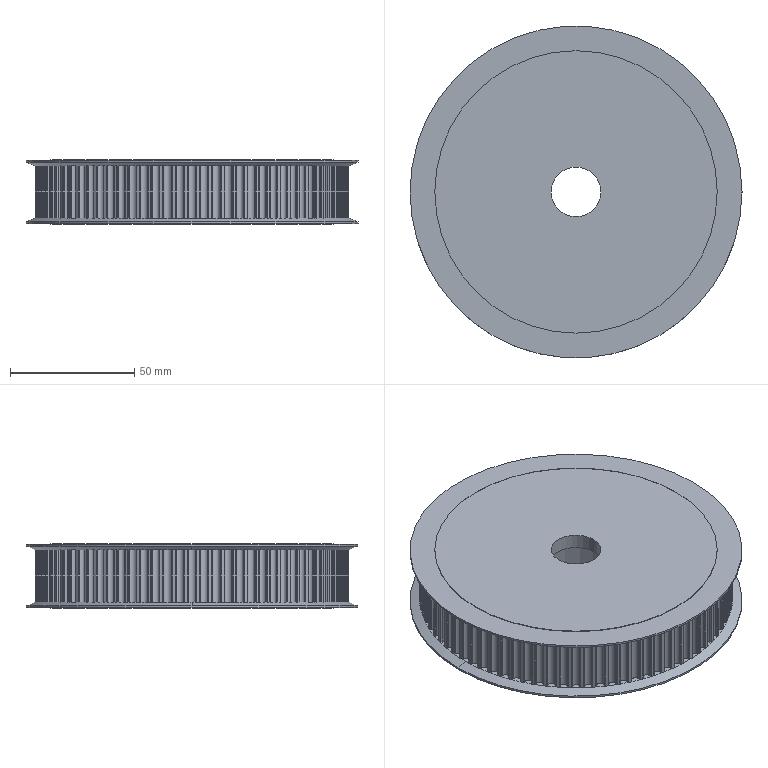Part | SolidWorks | features ICE 2, CirPattern 1, Cut 1, RefAxis 1, Revolution 1 | 1 solid | 736 faces | box 133.771 x 133.771 x 26 mm | volume 282633 mm3 | cylinder 407 | plane 325 | cone 4 | commonest cylinder face diameters 0.5 x198 3.143 x117 126.211 x80 113.771 x4 133.771 x4 20 x2